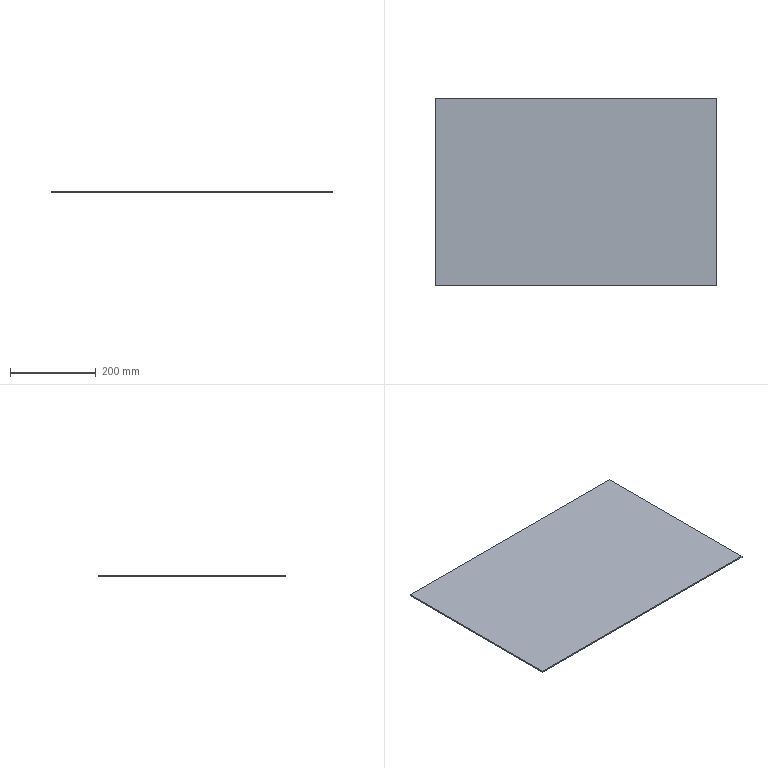Part | STEP file | 09-21 counterweight plate | 1 solid | 6 faces | box 658 x 438 x 3 mm | volume 864612 mm3 | plane 6
STEP:
#1=CARTESIAN_POINT('',(329.,-219.,0.));
#2=VERTEX_POINT('',#1);
#3=CARTESIAN_POINT('',(329.,219.,0.));
#4=VERTEX_POINT('',#3);
#5=CARTESIAN_POINT('',(329.,219.,0.));
#6=DIRECTION('',(0.,1.,0.));
#7=VECTOR('',#6,1000.);
#8=LINE('',#5,#7);
#9=EDGE_CURVE('',#2,#4,#8,.T.);
#10=ORIENTED_EDGE('',*,*,#9,.T.);
#11=CARTESIAN_POINT('',(329.,219.,3.));
#12=VERTEX_POINT('',#11);
#13=CARTESIAN_POINT('',(329.,219.,3.));
#14=DIRECTION('',(0.,0.,-1.));
#15=VECTOR('',#14,1000.);
#16=LINE('',#13,#15);
#17=EDGE_CURVE('',#12,#4,#16,.T.);
#18=ORIENTED_EDGE('',*,*,#17,.F.);
#19=CARTESIAN_POINT('',(329.,-219.,3.));
#20=VERTEX_POINT('',#19);
#21=CARTESIAN_POINT('',(329.,219.,3.));
#22=DIRECTION('',(0.,1.,0.));
#23=VECTOR('',#22,1000.);
#24=LINE('',#21,#23);
#25=EDGE_CURVE('',#20,#12,#24,.T.);
#26=ORIENTED_EDGE('',*,*,#25,.F.);
#27=CARTESIAN_POINT('',(329.,-219.,3.));
#28=DIRECTION('',(0.,0.,-1.));
#29=VECTOR('',#28,1000.);
#30=LINE('',#27,#29);
#31=EDGE_CURVE('',#20,#2,#30,.T.);
#32=ORIENTED_EDGE('',*,*,#31,.T.);
#33=EDGE_LOOP('',(#10,#18,#26,#32));
#34=FACE_OUTER_BOUND('',#33,.T.);
#35=CARTESIAN_POINT('',(329.,219.,3.));
#36=DIRECTION('',(-1.,0.,0.));
#37=DIRECTION('',(0.,0.,1.));
#38=AXIS2_PLACEMENT_3D('',#35,#36,#37);
#39=PLANE('',#38);
#40=ADVANCED_FACE('',(#34),#39,.F.);
#41=CARTESIAN_POINT('',(-329.,219.,0.));
#42=VERTEX_POINT('',#41);
#43=CARTESIAN_POINT('',(-329.,219.,0.));
#44=DIRECTION('',(-1.,0.,0.));
#45=VECTOR('',#44,1000.);
#46=LINE('',#43,#45);
#47=EDGE_CURVE('',#4,#42,#46,.T.);
#48=ORIENTED_EDGE('',*,*,#47,.T.);
#49=CARTESIAN_POINT('',(-329.,219.,3.));
#50=VERTEX_POINT('',#49);
#51=CARTESIAN_POINT('',(-329.,219.,3.));
#52=DIRECTION('',(0.,0.,-1.));
#53=VECTOR('',#52,1000.);
#54=LINE('',#51,#53);
#55=EDGE_CURVE('',#50,#42,#54,.T.);
#56=ORIENTED_EDGE('',*,*,#55,.F.);
#57=CARTESIAN_POINT('',(-329.,219.,3.));
#58=DIRECTION('',(-1.,0.,0.));
#59=VECTOR('',#58,1000.);
#60=LINE('',#57,#59);
#61=EDGE_CURVE('',#12,#50,#60,.T.);
#62=ORIENTED_EDGE('',*,*,#61,.F.);
#63=ORIENTED_EDGE('',*,*,#17,.T.);
#64=EDGE_LOOP('',(#48,#56,#62,#63));
#65=FACE_OUTER_BOUND('',#64,.T.);
#66=CARTESIAN_POINT('',(-329.,219.,3.));
#67=DIRECTION('',(0.,-1.,0.));
#68=DIRECTION('',(0.,0.,-1.));
#69=AXIS2_PLACEMENT_3D('',#66,#67,#68);
#70=PLANE('',#69);
#71=ADVANCED_FACE('',(#65),#70,.F.);
#72=CARTESIAN_POINT('',(-329.,-219.,0.));
#73=VERTEX_POINT('',#72);
#74=CARTESIAN_POINT('',(-329.,219.,0.));
#75=DIRECTION('',(0.,-1.,0.));
#76=VECTOR('',#75,1000.);
#77=LINE('',#74,#76);
#78=EDGE_CURVE('',#42,#73,#77,.T.);
#79=ORIENTED_EDGE('',*,*,#78,.T.);
#80=CARTESIAN_POINT('',(-329.,-219.,3.));
#81=VERTEX_POINT('',#80);
#82=CARTESIAN_POINT('',(-329.,-219.,3.));
#83=DIRECTION('',(0.,0.,-1.));
#84=VECTOR('',#83,1000.);
#85=LINE('',#82,#84);
#86=EDGE_CURVE('',#81,#73,#85,.T.);
#87=ORIENTED_EDGE('',*,*,#86,.F.);
#88=CARTESIAN_POINT('',(-329.,219.,3.));
#89=DIRECTION('',(0.,-1.,0.));
#90=VECTOR('',#89,1000.);
#91=LINE('',#88,#90);
#92=EDGE_CURVE('',#50,#81,#91,.T.);
#93=ORIENTED_EDGE('',*,*,#92,.F.);
#94=ORIENTED_EDGE('',*,*,#55,.T.);
#95=EDGE_LOOP('',(#79,#87,#93,#94));
#96=FACE_OUTER_BOUND('',#95,.T.);
#97=CARTESIAN_POINT('',(-329.,219.,3.));
#98=DIRECTION('',(1.,0.,0.));
#99=DIRECTION('',(0.,1.,0.));
#100=AXIS2_PLACEMENT_3D('',#97,#98,#99);
#101=PLANE('',#100);
#102=ADVANCED_FACE('',(#96),#101,.F.);
#103=CARTESIAN_POINT('',(-329.,-219.,0.));
#104=DIRECTION('',(1.,0.,0.));
#105=VECTOR('',#104,1000.);
#106=LINE('',#103,#105);
#107=EDGE_CURVE('',#73,#2,#106,.T.);
#108=ORIENTED_EDGE('',*,*,#107,.T.);
#109=ORIENTED_EDGE('',*,*,#31,.F.);
#110=CARTESIAN_POINT('',(-329.,-219.,3.));
#111=DIRECTION('',(1.,0.,0.));
#112=VECTOR('',#111,1000.);
#113=LINE('',#110,#112);
#114=EDGE_CURVE('',#81,#20,#113,.T.);
#115=ORIENTED_EDGE('',*,*,#114,.F.);
#116=ORIENTED_EDGE('',*,*,#86,.T.);
#117=EDGE_LOOP('',(#108,#109,#115,#116));
#118=FACE_OUTER_BOUND('',#117,.T.);
#119=CARTESIAN_POINT('',(-329.,-219.,3.));
#120=DIRECTION('',(0.,1.,0.));
#121=DIRECTION('',(0.,0.,1.));
#122=AXIS2_PLACEMENT_3D('',#119,#120,#121);
#123=PLANE('',#122);
#124=ADVANCED_FACE('',(#118),#123,.F.);
#125=ORIENTED_EDGE('',*,*,#25,.T.);
#126=ORIENTED_EDGE('',*,*,#61,.T.);
#127=ORIENTED_EDGE('',*,*,#92,.T.);
#128=ORIENTED_EDGE('',*,*,#114,.T.);
#129=EDGE_LOOP('',(#125,#126,#127,#128));
#130=FACE_OUTER_BOUND('',#129,.T.);
#131=CARTESIAN_POINT('',(329.,-219.,3.));
#132=DIRECTION('',(0.,0.,1.));
#133=DIRECTION('',(1.,0.,0.));
#134=AXIS2_PLACEMENT_3D('',#131,#132,#133);
#135=PLANE('',#134);
#136=ADVANCED_FACE('',(#130),#135,.T.);
#137=ORIENTED_EDGE('',*,*,#9,.F.);
#138=ORIENTED_EDGE('',*,*,#107,.F.);
#139=ORIENTED_EDGE('',*,*,#78,.F.);
#140=ORIENTED_EDGE('',*,*,#47,.F.);
#141=EDGE_LOOP('',(#137,#138,#139,#140));
#142=FACE_OUTER_BOUND('',#141,.T.);
#143=CARTESIAN_POINT('',(329.,-219.,0.));
#144=DIRECTION('',(0.,0.,1.));
#145=DIRECTION('',(1.,0.,0.));
#146=AXIS2_PLACEMENT_3D('',#143,#144,#145);
#147=PLANE('',#146);
#148=ADVANCED_FACE('',(#142),#147,.F.);
#149=CLOSED_SHELL('',(#40,#71,#102,#124,#136,#148));
#150=MANIFOLD_SOLID_BREP('',#149);
#151=CARTESIAN_POINT('',(0.,0.,0.));
#152=DIRECTION('',(0.,0.,1.));
#153=DIRECTION('',(1.,0.,0.));
#154=AXIS2_PLACEMENT_3D('',#151,#152,#153);
#155=(LENGTH_UNIT()NAMED_UNIT(*)SI_UNIT(.MILLI.,.METRE.));
#156=UNCERTAINTY_MEASURE_WITH_UNIT(LENGTH_MEASURE(0.00001),#155,'','');
#157=(NAMED_UNIT(*)PLANE_ANGLE_UNIT()SI_UNIT($,.RADIAN.));
#158=(NAMED_UNIT(*)SI_UNIT($,.STERADIAN.)SOLID_ANGLE_UNIT());
#159=(GEOMETRIC_REPRESENTATION_CONTEXT(3)GLOBAL_UNCERTAINTY_ASSIGNED_CONTEXT((#156))GLOBAL_UNIT_ASSIGNED_CONTEXT((#155,#157,#158))REPRESENTATION_CONTEXT('',''));
#160=ADVANCED_BREP_SHAPE_REPRESENTATION('',(#150,#154),#159);